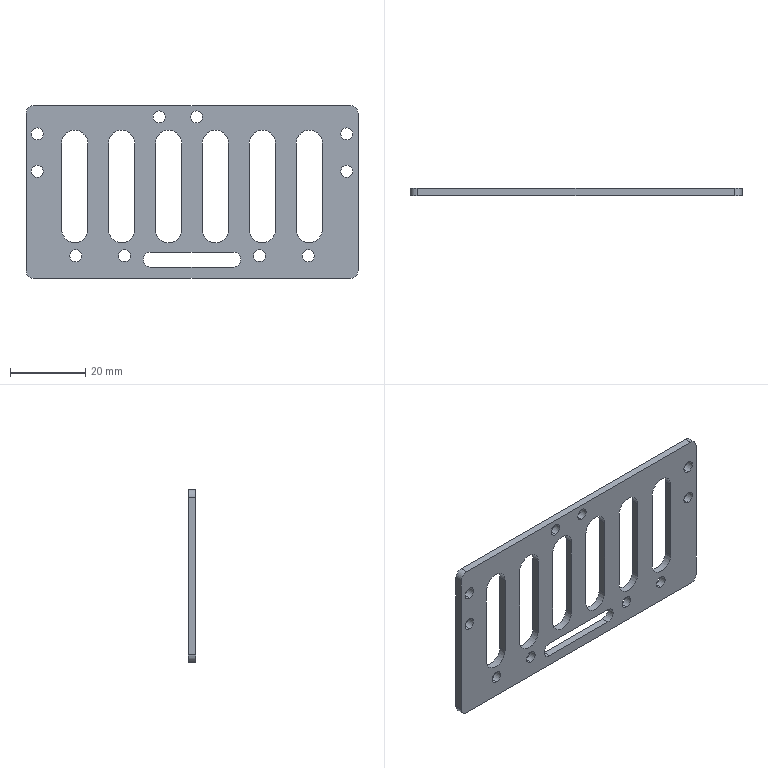Part | SolidWorks | features Extrusion 1, Fillet 1, ICE 1 | 1 solid | 64 faces | box 88.5 x 2 x 46 mm | volume 5379 mm3 | cylinder 44 | plane 20 | commonest cylinder face diameters 3.2 x20 7 x18 4 x6